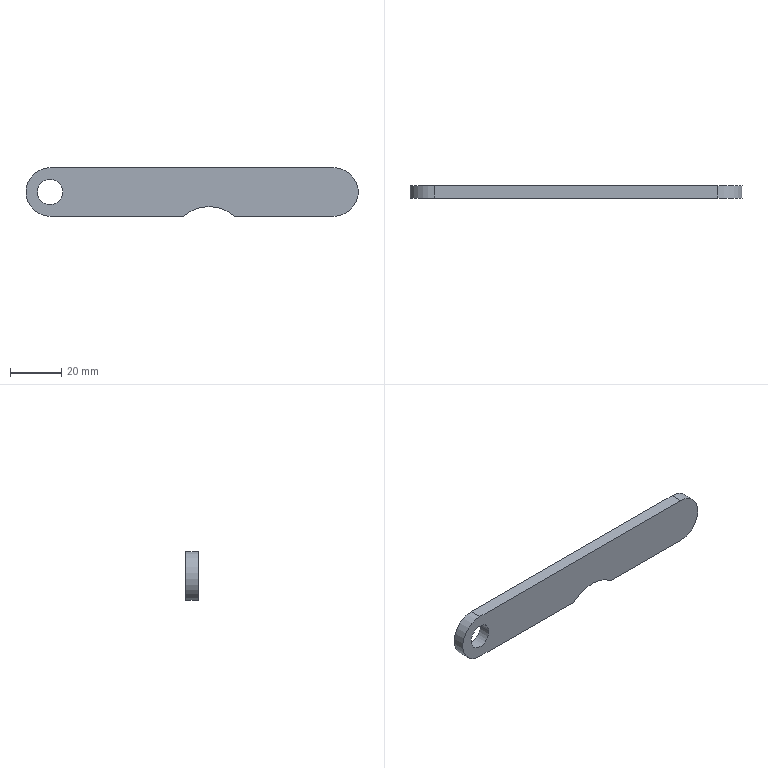Part | NX | features BREP 1 | 1 solid | 10 faces | box 130.175 x 4.763 x 19.05 mm | volume 10822 mm3 | plane 5 | cylinder 5 | commonest cylinder face diameters 9.906 x2 19.05 x2 30.48 x1
STEP:
#1=CARTESIAN_POINT('',(111.125,-4.763,-9.525));
#2=VERTEX_POINT('',#1);
#3=CARTESIAN_POINT('',(72.31,-4.763,-9.525));
#4=VERTEX_POINT('',#3);
#5=CARTESIAN_POINT('',(111.125,-4.763,-9.525));
#6=DIRECTION('',(-1.,0.,0.));
#7=VECTOR('',#6,1000.);
#8=LINE('',#5,#7);
#9=EDGE_CURVE('',#2,#4,#8,.T.);
#10=ORIENTED_EDGE('',*,*,#9,.F.);
#11=CARTESIAN_POINT('',(111.125,-4.763,9.525));
#12=VERTEX_POINT('',#11);
#13=CARTESIAN_POINT('',(111.125,-4.763,0.));
#14=DIRECTION('',(0.,1.,0.));
#15=DIRECTION('',(0.,0.,1.));
#16=AXIS2_PLACEMENT_3D('',#13,#14,#15);
#17=CIRCLE('',#16,9.525);
#18=EDGE_CURVE('',#12,#2,#17,.T.);
#19=ORIENTED_EDGE('',*,*,#18,.F.);
#20=CARTESIAN_POINT('',(0.,-4.763,9.525));
#21=VERTEX_POINT('',#20);
#22=CARTESIAN_POINT('',(0.,-4.763,9.525));
#23=DIRECTION('',(1.,0.,0.));
#24=VECTOR('',#23,1000.);
#25=LINE('',#22,#24);
#26=EDGE_CURVE('',#21,#12,#25,.T.);
#27=ORIENTED_EDGE('',*,*,#26,.F.);
#28=CARTESIAN_POINT('',(0.,-4.763,-9.525));
#29=VERTEX_POINT('',#28);
#30=CARTESIAN_POINT('',(0.,-4.763,0.));
#31=DIRECTION('',(0.,1.,0.));
#32=DIRECTION('',(0.,0.,-1.));
#33=AXIS2_PLACEMENT_3D('',#30,#31,#32);
#34=CIRCLE('',#33,9.525);
#35=EDGE_CURVE('',#29,#21,#34,.T.);
#36=ORIENTED_EDGE('',*,*,#35,.F.);
#37=CARTESIAN_POINT('',(52.15,-4.763,-9.525));
#38=VERTEX_POINT('',#37);
#39=CARTESIAN_POINT('',(52.15,-4.763,-9.525));
#40=DIRECTION('',(-1.,0.,0.));
#41=VECTOR('',#40,1000.);
#42=LINE('',#39,#41);
#43=EDGE_CURVE('',#38,#29,#42,.T.);
#44=ORIENTED_EDGE('',*,*,#43,.F.);
#45=CARTESIAN_POINT('',(62.23,-4.763,-20.955));
#46=DIRECTION('',(0.,-1.,0.));
#47=DIRECTION('',(0.6614,0.,0.75));
#48=AXIS2_PLACEMENT_3D('',#45,#46,#47);
#49=CIRCLE('',#48,15.24);
#50=EDGE_CURVE('',#4,#38,#49,.T.);
#51=ORIENTED_EDGE('',*,*,#50,.F.);
#52=EDGE_LOOP('',(#10,#19,#27,#36,#44,#51));
#53=FACE_BOUND('',#52,.T.);
#54=CARTESIAN_POINT('',(4.953,-4.763,0.));
#55=VERTEX_POINT('',#54);
#56=CARTESIAN_POINT('',(-4.953,-4.763,0.));
#57=VERTEX_POINT('',#56);
#58=CARTESIAN_POINT('',(0.,-4.763,0.));
#59=DIRECTION('',(0.,1.,0.));
#60=DIRECTION('',(1.,0.,0.));
#61=AXIS2_PLACEMENT_3D('',#58,#59,#60);
#62=CIRCLE('',#61,4.953);
#63=EDGE_CURVE('',#55,#57,#62,.T.);
#64=ORIENTED_EDGE('',*,*,#63,.T.);
#65=CARTESIAN_POINT('',(0.,-4.763,0.));
#66=DIRECTION('',(0.,1.,0.));
#67=DIRECTION('',(-1.,0.,0.));
#68=AXIS2_PLACEMENT_3D('',#65,#66,#67);
#69=CIRCLE('',#68,4.953);
#70=EDGE_CURVE('',#57,#55,#69,.T.);
#71=ORIENTED_EDGE('',*,*,#70,.T.);
#72=EDGE_LOOP('',(#64,#71));
#73=FACE_BOUND('',#72,.T.);
#74=CARTESIAN_POINT('',(0.,-4.763,0.));
#75=DIRECTION('',(0.,1.,0.));
#76=DIRECTION('',(1.,0.,0.));
#77=AXIS2_PLACEMENT_3D('',#74,#75,#76);
#78=PLANE('',#77);
#79=ADVANCED_FACE('',(#53,#73),#78,.F.);
#80=CARTESIAN_POINT('',(4.953,0.,0.));
#81=VERTEX_POINT('',#80);
#82=CARTESIAN_POINT('',(4.953,0.,0.));
#83=DIRECTION('',(0.,-1.,0.));
#84=VECTOR('',#83,1000.);
#85=LINE('',#82,#84);
#86=EDGE_CURVE('',#55,#81,#85,.F.);
#87=ORIENTED_EDGE('',*,*,#86,.F.);
#88=ORIENTED_EDGE('',*,*,#70,.F.);
#89=CARTESIAN_POINT('',(-4.953,0.,0.));
#90=VERTEX_POINT('',#89);
#91=CARTESIAN_POINT('',(-4.953,0.,0.));
#92=DIRECTION('',(0.,-1.,0.));
#93=VECTOR('',#92,1000.);
#94=LINE('',#91,#93);
#95=EDGE_CURVE('',#57,#90,#94,.F.);
#96=ORIENTED_EDGE('',*,*,#95,.T.);
#97=CARTESIAN_POINT('',(0.,0.,0.));
#98=DIRECTION('',(0.,1.,0.));
#99=DIRECTION('',(-1.,0.,0.));
#100=AXIS2_PLACEMENT_3D('',#97,#98,#99);
#101=CIRCLE('',#100,4.953);
#102=EDGE_CURVE('',#90,#81,#101,.T.);
#103=ORIENTED_EDGE('',*,*,#102,.T.);
#104=EDGE_LOOP('',(#87,#88,#96,#103));
#105=FACE_BOUND('',#104,.T.);
#106=CARTESIAN_POINT('',(0.,-2.381,0.));
#107=DIRECTION('',(0.,1.,0.));
#108=DIRECTION('',(-1.,0.,0.));
#109=AXIS2_PLACEMENT_3D('',#106,#107,#108);
#110=CYLINDRICAL_SURFACE('',#109,4.953);
#111=ADVANCED_FACE('',(#105),#110,.F.);
#112=CARTESIAN_POINT('',(52.15,0.,-9.525));
#113=VERTEX_POINT('',#112);
#114=CARTESIAN_POINT('',(0.,0.,-9.525));
#115=VERTEX_POINT('',#114);
#116=CARTESIAN_POINT('',(52.15,0.,-9.525));
#117=DIRECTION('',(-1.,0.,0.));
#118=VECTOR('',#117,1000.);
#119=LINE('',#116,#118);
#120=EDGE_CURVE('',#113,#115,#119,.T.);
#121=ORIENTED_EDGE('',*,*,#120,.T.);
#122=CARTESIAN_POINT('',(0.,0.,9.525));
#123=VERTEX_POINT('',#122);
#124=CARTESIAN_POINT('',(0.,0.,0.));
#125=DIRECTION('',(0.,1.,0.));
#126=DIRECTION('',(0.,0.,-1.));
#127=AXIS2_PLACEMENT_3D('',#124,#125,#126);
#128=CIRCLE('',#127,9.525);
#129=EDGE_CURVE('',#115,#123,#128,.T.);
#130=ORIENTED_EDGE('',*,*,#129,.T.);
#131=CARTESIAN_POINT('',(111.125,0.,9.525));
#132=VERTEX_POINT('',#131);
#133=CARTESIAN_POINT('',(0.,0.,9.525));
#134=DIRECTION('',(1.,0.,0.));
#135=VECTOR('',#134,1000.);
#136=LINE('',#133,#135);
#137=EDGE_CURVE('',#123,#132,#136,.T.);
#138=ORIENTED_EDGE('',*,*,#137,.T.);
#139=CARTESIAN_POINT('',(111.125,0.,-9.525));
#140=VERTEX_POINT('',#139);
#141=CARTESIAN_POINT('',(111.125,0.,0.));
#142=DIRECTION('',(0.,1.,0.));
#143=DIRECTION('',(0.,0.,1.));
#144=AXIS2_PLACEMENT_3D('',#141,#142,#143);
#145=CIRCLE('',#144,9.525);
#146=EDGE_CURVE('',#132,#140,#145,.T.);
#147=ORIENTED_EDGE('',*,*,#146,.T.);
#148=CARTESIAN_POINT('',(72.31,0.,-9.525));
#149=VERTEX_POINT('',#148);
#150=CARTESIAN_POINT('',(111.125,0.,-9.525));
#151=DIRECTION('',(-1.,0.,0.));
#152=VECTOR('',#151,1000.);
#153=LINE('',#150,#152);
#154=EDGE_CURVE('',#140,#149,#153,.T.);
#155=ORIENTED_EDGE('',*,*,#154,.T.);
#156=CARTESIAN_POINT('',(62.23,0.,-20.955));
#157=DIRECTION('',(0.,-1.,0.));
#158=DIRECTION('',(0.6614,0.,0.75));
#159=AXIS2_PLACEMENT_3D('',#156,#157,#158);
#160=CIRCLE('',#159,15.24);
#161=EDGE_CURVE('',#149,#113,#160,.T.);
#162=ORIENTED_EDGE('',*,*,#161,.T.);
#163=EDGE_LOOP('',(#121,#130,#138,#147,#155,#162));
#164=FACE_BOUND('',#163,.T.);
#165=CARTESIAN_POINT('',(0.,0.,0.));
#166=DIRECTION('',(0.,1.,0.));
#167=DIRECTION('',(1.,0.,0.));
#168=AXIS2_PLACEMENT_3D('',#165,#166,#167);
#169=CIRCLE('',#168,4.953);
#170=EDGE_CURVE('',#81,#90,#169,.T.);
#171=ORIENTED_EDGE('',*,*,#170,.F.);
#172=ORIENTED_EDGE('',*,*,#102,.F.);
#173=EDGE_LOOP('',(#171,#172));
#174=FACE_BOUND('',#173,.T.);
#175=CARTESIAN_POINT('',(0.,0.,0.));
#176=DIRECTION('',(0.,1.,0.));
#177=DIRECTION('',(1.,0.,0.));
#178=AXIS2_PLACEMENT_3D('',#175,#176,#177);
#179=PLANE('',#178);
#180=ADVANCED_FACE('',(#164,#174),#179,.T.);
#181=ORIENTED_EDGE('',*,*,#95,.F.);
#182=ORIENTED_EDGE('',*,*,#63,.F.);
#183=ORIENTED_EDGE('',*,*,#86,.T.);
#184=ORIENTED_EDGE('',*,*,#170,.T.);
#185=EDGE_LOOP('',(#181,#182,#183,#184));
#186=FACE_BOUND('',#185,.T.);
#187=CARTESIAN_POINT('',(0.,-2.381,0.));
#188=DIRECTION('',(0.,1.,0.));
#189=DIRECTION('',(1.,0.,0.));
#190=AXIS2_PLACEMENT_3D('',#187,#188,#189);
#191=CYLINDRICAL_SURFACE('',#190,4.953);
#192=ADVANCED_FACE('',(#186),#191,.F.);
#193=CARTESIAN_POINT('',(52.15,-4.763,-9.525));
#194=DIRECTION('',(0.,1.,0.));
#195=VECTOR('',#194,1000.);
#196=LINE('',#193,#195);
#197=EDGE_CURVE('',#38,#113,#196,.T.);
#198=ORIENTED_EDGE('',*,*,#197,.T.);
#199=ORIENTED_EDGE('',*,*,#161,.F.);
#200=CARTESIAN_POINT('',(72.31,-4.763,-9.525));
#201=DIRECTION('',(0.,1.,0.));
#202=VECTOR('',#201,1000.);
#203=LINE('',#200,#202);
#204=EDGE_CURVE('',#4,#149,#203,.T.);
#205=ORIENTED_EDGE('',*,*,#204,.F.);
#206=ORIENTED_EDGE('',*,*,#50,.T.);
#207=EDGE_LOOP('',(#198,#199,#205,#206));
#208=FACE_BOUND('',#207,.T.);
#209=CARTESIAN_POINT('',(62.23,-2.381,-20.955));
#210=DIRECTION('',(0.,-1.,0.));
#211=DIRECTION('',(0.6614,0.,0.75));
#212=AXIS2_PLACEMENT_3D('',#209,#210,#211);
#213=CYLINDRICAL_SURFACE('',#212,15.24);
#214=ADVANCED_FACE('',(#208),#213,.F.);
#215=ORIENTED_EDGE('',*,*,#43,.T.);
#216=CARTESIAN_POINT('',(0.,0.,-9.525));
#217=DIRECTION('',(0.,-1.,0.));
#218=VECTOR('',#217,1000.);
#219=LINE('',#216,#218);
#220=EDGE_CURVE('',#115,#29,#219,.T.);
#221=ORIENTED_EDGE('',*,*,#220,.F.);
#222=ORIENTED_EDGE('',*,*,#120,.F.);
#223=ORIENTED_EDGE('',*,*,#197,.F.);
#224=EDGE_LOOP('',(#215,#221,#222,#223));
#225=FACE_BOUND('',#224,.T.);
#226=CARTESIAN_POINT('',(55.562,-2.381,-9.525));
#227=DIRECTION('',(0.,0.,-1.));
#228=DIRECTION('',(0.,-1.,0.));
#229=AXIS2_PLACEMENT_3D('',#226,#227,#228);
#230=PLANE('',#229);
#231=ADVANCED_FACE('',(#225),#230,.T.);
#232=ORIENTED_EDGE('',*,*,#154,.F.);
#233=CARTESIAN_POINT('',(111.125,0.,-9.525));
#234=DIRECTION('',(0.,-1.,0.));
#235=VECTOR('',#234,1000.);
#236=LINE('',#233,#235);
#237=EDGE_CURVE('',#140,#2,#236,.T.);
#238=ORIENTED_EDGE('',*,*,#237,.T.);
#239=ORIENTED_EDGE('',*,*,#9,.T.);
#240=ORIENTED_EDGE('',*,*,#204,.T.);
#241=EDGE_LOOP('',(#232,#238,#239,#240));
#242=FACE_BOUND('',#241,.T.);
#243=CARTESIAN_POINT('',(55.562,-2.381,-9.525));
#244=DIRECTION('',(0.,0.,-1.));
#245=DIRECTION('',(0.,-1.,0.));
#246=AXIS2_PLACEMENT_3D('',#243,#244,#245);
#247=PLANE('',#246);
#248=ADVANCED_FACE('',(#242),#247,.T.);
#249=ORIENTED_EDGE('',*,*,#220,.T.);
#250=ORIENTED_EDGE('',*,*,#35,.T.);
#251=CARTESIAN_POINT('',(0.,0.,9.525));
#252=DIRECTION('',(0.,-1.,0.));
#253=VECTOR('',#252,1000.);
#254=LINE('',#251,#253);
#255=EDGE_CURVE('',#123,#21,#254,.T.);
#256=ORIENTED_EDGE('',*,*,#255,.F.);
#257=ORIENTED_EDGE('',*,*,#129,.F.);
#258=EDGE_LOOP('',(#249,#250,#256,#257));
#259=FACE_BOUND('',#258,.T.);
#260=CARTESIAN_POINT('',(0.,-2.381,0.));
#261=DIRECTION('',(0.,1.,0.));
#262=DIRECTION('',(0.,0.,-1.));
#263=AXIS2_PLACEMENT_3D('',#260,#261,#262);
#264=CYLINDRICAL_SURFACE('',#263,9.525);
#265=ADVANCED_FACE('',(#259),#264,.T.);
#266=ORIENTED_EDGE('',*,*,#255,.T.);
#267=ORIENTED_EDGE('',*,*,#26,.T.);
#268=CARTESIAN_POINT('',(111.125,0.,9.525));
#269=DIRECTION('',(0.,-1.,0.));
#270=VECTOR('',#269,1000.);
#271=LINE('',#268,#270);
#272=EDGE_CURVE('',#132,#12,#271,.T.);
#273=ORIENTED_EDGE('',*,*,#272,.F.);
#274=ORIENTED_EDGE('',*,*,#137,.F.);
#275=EDGE_LOOP('',(#266,#267,#273,#274));
#276=FACE_BOUND('',#275,.T.);
#277=CARTESIAN_POINT('',(55.562,-2.381,9.525));
#278=DIRECTION('',(0.,0.,1.));
#279=DIRECTION('',(1.,0.,0.));
#280=AXIS2_PLACEMENT_3D('',#277,#278,#279);
#281=PLANE('',#280);
#282=ADVANCED_FACE('',(#276),#281,.T.);
#283=ORIENTED_EDGE('',*,*,#272,.T.);
#284=ORIENTED_EDGE('',*,*,#18,.T.);
#285=ORIENTED_EDGE('',*,*,#237,.F.);
#286=ORIENTED_EDGE('',*,*,#146,.F.);
#287=EDGE_LOOP('',(#283,#284,#285,#286));
#288=FACE_BOUND('',#287,.T.);
#289=CARTESIAN_POINT('',(111.125,-2.381,0.));
#290=DIRECTION('',(0.,1.,0.));
#291=DIRECTION('',(0.,0.,1.));
#292=AXIS2_PLACEMENT_3D('',#289,#290,#291);
#293=CYLINDRICAL_SURFACE('',#292,9.525);
#294=ADVANCED_FACE('',(#288),#293,.T.);
#295=CLOSED_SHELL('',(#79,#111,#180,#192,#214,#231,#248,#265,#282,#294));
#296=MANIFOLD_SOLID_BREP('',#295);
#297=(LENGTH_UNIT()NAMED_UNIT(*)SI_UNIT(.MILLI.,.METRE.));
#298=UNCERTAINTY_MEASURE_WITH_UNIT(LENGTH_MEASURE(0.00001),#297,'','');
#299=(NAMED_UNIT(*)PLANE_ANGLE_UNIT()SI_UNIT($,.RADIAN.));
#300=(NAMED_UNIT(*)SI_UNIT($,.STERADIAN.)SOLID_ANGLE_UNIT());
#301=(GEOMETRIC_REPRESENTATION_CONTEXT(3)GLOBAL_UNCERTAINTY_ASSIGNED_CONTEXT((#298))GLOBAL_UNIT_ASSIGNED_CONTEXT((#297,#299,#300))REPRESENTATION_CONTEXT('',''));
#302=ADVANCED_BREP_SHAPE_REPRESENTATION('',(#296),#301);